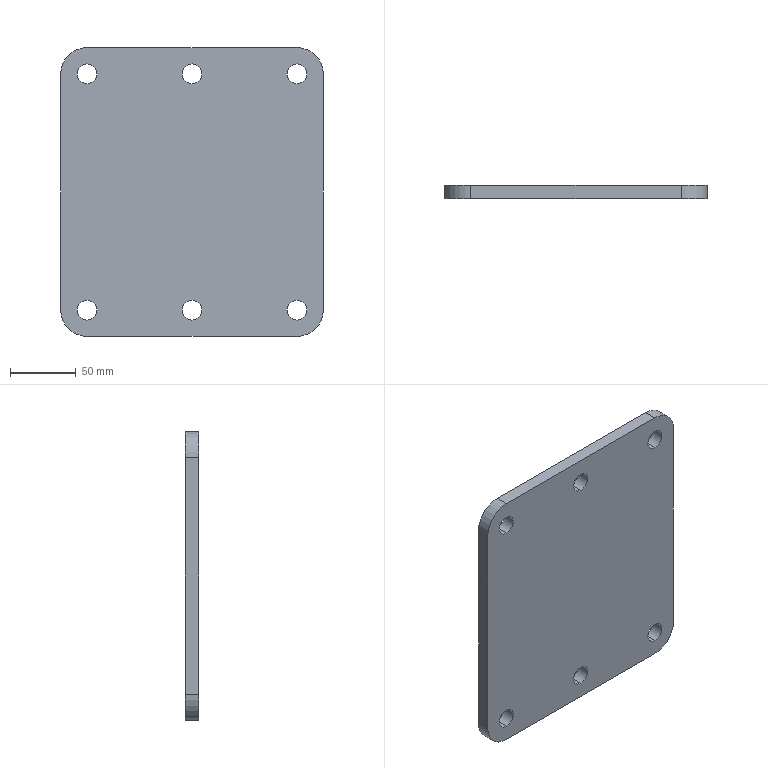Part | SolidWorks | features Extrusion 1, Fillet 1, ICE 1, LPattern 1 | 1 solid | 22 faces | box 200 x 10 x 220 mm | volume 425963 mm3 | cylinder 16 | plane 6 | commonest cylinder face diameters 15 x12 40 x4
STEP:
#1=CARTESIAN_POINT('',(80.,-5.,82.5));
#2=VERTEX_POINT('',#1);
#3=CARTESIAN_POINT('',(80.,-5.,97.5));
#4=VERTEX_POINT('',#3);
#5=CARTESIAN_POINT('',(80.,-5.,90.));
#6=DIRECTION('',(0.,1.,0.));
#7=DIRECTION('',(0.,0.,1.));
#8=AXIS2_PLACEMENT_3D('',#5,#6,#7);
#9=CIRCLE('',#8,7.5);
#10=EDGE_CURVE('',#2,#4,#9,.T.);
#11=ORIENTED_EDGE('',*,*,#10,.F.);
#12=CARTESIAN_POINT('',(80.,5.,82.5));
#13=VERTEX_POINT('',#12);
#14=CARTESIAN_POINT('',(80.,-5.,82.5));
#15=DIRECTION('',(0.,1.,0.));
#16=VECTOR('',#15,1000.);
#17=LINE('',#14,#16);
#18=EDGE_CURVE('',#2,#13,#17,.T.);
#19=ORIENTED_EDGE('',*,*,#18,.T.);
#20=CARTESIAN_POINT('',(80.,5.,97.5));
#21=VERTEX_POINT('',#20);
#22=CARTESIAN_POINT('',(80.,5.,90.));
#23=DIRECTION('',(0.,1.,0.));
#24=DIRECTION('',(0.,0.,1.));
#25=AXIS2_PLACEMENT_3D('',#22,#23,#24);
#26=CIRCLE('',#25,7.5);
#27=EDGE_CURVE('',#13,#21,#26,.T.);
#28=ORIENTED_EDGE('',*,*,#27,.T.);
#29=CARTESIAN_POINT('',(80.,-5.,97.5));
#30=DIRECTION('',(0.,1.,0.));
#31=VECTOR('',#30,1000.);
#32=LINE('',#29,#31);
#33=EDGE_CURVE('',#4,#21,#32,.T.);
#34=ORIENTED_EDGE('',*,*,#33,.F.);
#35=EDGE_LOOP('',(#11,#19,#28,#34));
#36=FACE_OUTER_BOUND('',#35,.T.);
#37=CARTESIAN_POINT('',(80.,-5.,90.));
#38=DIRECTION('',(0.,1.,0.));
#39=DIRECTION('',(0.,0.,1.));
#40=AXIS2_PLACEMENT_3D('',#37,#38,#39);
#41=CYLINDRICAL_SURFACE('',#40,7.5);
#42=ADVANCED_FACE('',(#36),#41,.F.);
#43=CARTESIAN_POINT('',(80.,-5.,-97.5));
#44=VERTEX_POINT('',#43);
#45=CARTESIAN_POINT('',(80.,-5.,-82.5));
#46=VERTEX_POINT('',#45);
#47=CARTESIAN_POINT('',(80.,-5.,-90.));
#48=DIRECTION('',(0.,1.,0.));
#49=DIRECTION('',(0.,0.,1.));
#50=AXIS2_PLACEMENT_3D('',#47,#48,#49);
#51=CIRCLE('',#50,7.5);
#52=EDGE_CURVE('',#44,#46,#51,.T.);
#53=ORIENTED_EDGE('',*,*,#52,.F.);
#54=CARTESIAN_POINT('',(80.,5.,-97.5));
#55=VERTEX_POINT('',#54);
#56=CARTESIAN_POINT('',(80.,-5.,-97.5));
#57=DIRECTION('',(0.,1.,0.));
#58=VECTOR('',#57,1000.);
#59=LINE('',#56,#58);
#60=EDGE_CURVE('',#44,#55,#59,.T.);
#61=ORIENTED_EDGE('',*,*,#60,.T.);
#62=CARTESIAN_POINT('',(80.,5.,-82.5));
#63=VERTEX_POINT('',#62);
#64=CARTESIAN_POINT('',(80.,5.,-90.));
#65=DIRECTION('',(0.,1.,0.));
#66=DIRECTION('',(0.,0.,1.));
#67=AXIS2_PLACEMENT_3D('',#64,#65,#66);
#68=CIRCLE('',#67,7.5);
#69=EDGE_CURVE('',#55,#63,#68,.T.);
#70=ORIENTED_EDGE('',*,*,#69,.T.);
#71=CARTESIAN_POINT('',(80.,-5.,-82.5));
#72=DIRECTION('',(0.,1.,0.));
#73=VECTOR('',#72,1000.);
#74=LINE('',#71,#73);
#75=EDGE_CURVE('',#46,#63,#74,.T.);
#76=ORIENTED_EDGE('',*,*,#75,.F.);
#77=EDGE_LOOP('',(#53,#61,#70,#76));
#78=FACE_OUTER_BOUND('',#77,.T.);
#79=CARTESIAN_POINT('',(80.,-5.,-90.));
#80=DIRECTION('',(0.,1.,0.));
#81=DIRECTION('',(0.,0.,1.));
#82=AXIS2_PLACEMENT_3D('',#79,#80,#81);
#83=CYLINDRICAL_SURFACE('',#82,7.5);
#84=ADVANCED_FACE('',(#78),#83,.F.);
#85=CARTESIAN_POINT('',(0.,-5.,-97.5));
#86=VERTEX_POINT('',#85);
#87=CARTESIAN_POINT('',(0.,-5.,-82.5));
#88=VERTEX_POINT('',#87);
#89=CARTESIAN_POINT('',(0.,-5.,-90.));
#90=DIRECTION('',(0.,1.,0.));
#91=DIRECTION('',(0.,0.,1.));
#92=AXIS2_PLACEMENT_3D('',#89,#90,#91);
#93=CIRCLE('',#92,7.5);
#94=EDGE_CURVE('',#86,#88,#93,.T.);
#95=ORIENTED_EDGE('',*,*,#94,.F.);
#96=CARTESIAN_POINT('',(0.,5.,-97.5));
#97=VERTEX_POINT('',#96);
#98=CARTESIAN_POINT('',(0.,-5.,-97.5));
#99=DIRECTION('',(0.,1.,0.));
#100=VECTOR('',#99,1000.);
#101=LINE('',#98,#100);
#102=EDGE_CURVE('',#86,#97,#101,.T.);
#103=ORIENTED_EDGE('',*,*,#102,.T.);
#104=CARTESIAN_POINT('',(0.,5.,-82.5));
#105=VERTEX_POINT('',#104);
#106=CARTESIAN_POINT('',(0.,5.,-90.));
#107=DIRECTION('',(0.,1.,0.));
#108=DIRECTION('',(0.,0.,1.));
#109=AXIS2_PLACEMENT_3D('',#106,#107,#108);
#110=CIRCLE('',#109,7.5);
#111=EDGE_CURVE('',#97,#105,#110,.T.);
#112=ORIENTED_EDGE('',*,*,#111,.T.);
#113=CARTESIAN_POINT('',(0.,-5.,-82.5));
#114=DIRECTION('',(0.,1.,0.));
#115=VECTOR('',#114,1000.);
#116=LINE('',#113,#115);
#117=EDGE_CURVE('',#88,#105,#116,.T.);
#118=ORIENTED_EDGE('',*,*,#117,.F.);
#119=EDGE_LOOP('',(#95,#103,#112,#118));
#120=FACE_OUTER_BOUND('',#119,.T.);
#121=CARTESIAN_POINT('',(0.,-5.,-90.));
#122=DIRECTION('',(0.,1.,0.));
#123=DIRECTION('',(0.,0.,1.));
#124=AXIS2_PLACEMENT_3D('',#121,#122,#123);
#125=CYLINDRICAL_SURFACE('',#124,7.5);
#126=ADVANCED_FACE('',(#120),#125,.F.);
#127=CARTESIAN_POINT('',(0.,-5.,82.5));
#128=VERTEX_POINT('',#127);
#129=CARTESIAN_POINT('',(0.,-5.,97.5));
#130=VERTEX_POINT('',#129);
#131=CARTESIAN_POINT('',(0.,-5.,90.));
#132=DIRECTION('',(0.,1.,0.));
#133=DIRECTION('',(0.,0.,1.));
#134=AXIS2_PLACEMENT_3D('',#131,#132,#133);
#135=CIRCLE('',#134,7.5);
#136=EDGE_CURVE('',#128,#130,#135,.T.);
#137=ORIENTED_EDGE('',*,*,#136,.F.);
#138=CARTESIAN_POINT('',(0.,5.,82.5));
#139=VERTEX_POINT('',#138);
#140=CARTESIAN_POINT('',(0.,-5.,82.5));
#141=DIRECTION('',(0.,1.,0.));
#142=VECTOR('',#141,1000.);
#143=LINE('',#140,#142);
#144=EDGE_CURVE('',#128,#139,#143,.T.);
#145=ORIENTED_EDGE('',*,*,#144,.T.);
#146=CARTESIAN_POINT('',(0.,5.,97.5));
#147=VERTEX_POINT('',#146);
#148=CARTESIAN_POINT('',(0.,5.,90.));
#149=DIRECTION('',(0.,1.,0.));
#150=DIRECTION('',(0.,0.,1.));
#151=AXIS2_PLACEMENT_3D('',#148,#149,#150);
#152=CIRCLE('',#151,7.5);
#153=EDGE_CURVE('',#139,#147,#152,.T.);
#154=ORIENTED_EDGE('',*,*,#153,.T.);
#155=CARTESIAN_POINT('',(0.,-5.,97.5));
#156=DIRECTION('',(0.,1.,0.));
#157=VECTOR('',#156,1000.);
#158=LINE('',#155,#157);
#159=EDGE_CURVE('',#130,#147,#158,.T.);
#160=ORIENTED_EDGE('',*,*,#159,.F.);
#161=EDGE_LOOP('',(#137,#145,#154,#160));
#162=FACE_OUTER_BOUND('',#161,.T.);
#163=CARTESIAN_POINT('',(0.,-5.,90.));
#164=DIRECTION('',(0.,1.,0.));
#165=DIRECTION('',(0.,0.,1.));
#166=AXIS2_PLACEMENT_3D('',#163,#164,#165);
#167=CYLINDRICAL_SURFACE('',#166,7.5);
#168=ADVANCED_FACE('',(#162),#167,.F.);
#169=CARTESIAN_POINT('',(-80.,-5.,-97.5));
#170=VERTEX_POINT('',#169);
#171=CARTESIAN_POINT('',(-80.,-5.,-82.5));
#172=VERTEX_POINT('',#171);
#173=CARTESIAN_POINT('',(-80.,-5.,-90.));
#174=DIRECTION('',(0.,1.,0.));
#175=DIRECTION('',(0.,0.,1.));
#176=AXIS2_PLACEMENT_3D('',#173,#174,#175);
#177=CIRCLE('',#176,7.5);
#178=EDGE_CURVE('',#170,#172,#177,.T.);
#179=ORIENTED_EDGE('',*,*,#178,.F.);
#180=CARTESIAN_POINT('',(-80.,5.,-97.5));
#181=VERTEX_POINT('',#180);
#182=CARTESIAN_POINT('',(-80.,-5.,-97.5));
#183=DIRECTION('',(0.,1.,0.));
#184=VECTOR('',#183,1000.);
#185=LINE('',#182,#184);
#186=EDGE_CURVE('',#170,#181,#185,.T.);
#187=ORIENTED_EDGE('',*,*,#186,.T.);
#188=CARTESIAN_POINT('',(-80.,5.,-82.5));
#189=VERTEX_POINT('',#188);
#190=CARTESIAN_POINT('',(-80.,5.,-90.));
#191=DIRECTION('',(0.,1.,0.));
#192=DIRECTION('',(0.,0.,1.));
#193=AXIS2_PLACEMENT_3D('',#190,#191,#192);
#194=CIRCLE('',#193,7.5);
#195=EDGE_CURVE('',#181,#189,#194,.T.);
#196=ORIENTED_EDGE('',*,*,#195,.T.);
#197=CARTESIAN_POINT('',(-80.,-5.,-82.5));
#198=DIRECTION('',(0.,1.,0.));
#199=VECTOR('',#198,1000.);
#200=LINE('',#197,#199);
#201=EDGE_CURVE('',#172,#189,#200,.T.);
#202=ORIENTED_EDGE('',*,*,#201,.F.);
#203=EDGE_LOOP('',(#179,#187,#196,#202));
#204=FACE_OUTER_BOUND('',#203,.T.);
#205=CARTESIAN_POINT('',(-80.,-5.,-90.));
#206=DIRECTION('',(0.,1.,0.));
#207=DIRECTION('',(0.,0.,1.));
#208=AXIS2_PLACEMENT_3D('',#205,#206,#207);
#209=CYLINDRICAL_SURFACE('',#208,7.5);
#210=ADVANCED_FACE('',(#204),#209,.F.);
#211=CARTESIAN_POINT('',(-80.,-5.,82.5));
#212=VERTEX_POINT('',#211);
#213=CARTESIAN_POINT('',(-80.,-5.,97.5));
#214=VERTEX_POINT('',#213);
#215=CARTESIAN_POINT('',(-80.,-5.,90.));
#216=DIRECTION('',(0.,1.,0.));
#217=DIRECTION('',(0.,0.,1.));
#218=AXIS2_PLACEMENT_3D('',#215,#216,#217);
#219=CIRCLE('',#218,7.5);
#220=EDGE_CURVE('',#212,#214,#219,.T.);
#221=ORIENTED_EDGE('',*,*,#220,.F.);
#222=CARTESIAN_POINT('',(-80.,5.,82.5));
#223=VERTEX_POINT('',#222);
#224=CARTESIAN_POINT('',(-80.,-5.,82.5));
#225=DIRECTION('',(0.,1.,0.));
#226=VECTOR('',#225,1000.);
#227=LINE('',#224,#226);
#228=EDGE_CURVE('',#212,#223,#227,.T.);
#229=ORIENTED_EDGE('',*,*,#228,.T.);
#230=CARTESIAN_POINT('',(-80.,5.,97.5));
#231=VERTEX_POINT('',#230);
#232=CARTESIAN_POINT('',(-80.,5.,90.));
#233=DIRECTION('',(0.,1.,0.));
#234=DIRECTION('',(0.,0.,1.));
#235=AXIS2_PLACEMENT_3D('',#232,#233,#234);
#236=CIRCLE('',#235,7.5);
#237=EDGE_CURVE('',#223,#231,#236,.T.);
#238=ORIENTED_EDGE('',*,*,#237,.T.);
#239=CARTESIAN_POINT('',(-80.,-5.,97.5));
#240=DIRECTION('',(0.,1.,0.));
#241=VECTOR('',#240,1000.);
#242=LINE('',#239,#241);
#243=EDGE_CURVE('',#214,#231,#242,.T.);
#244=ORIENTED_EDGE('',*,*,#243,.F.);
#245=EDGE_LOOP('',(#221,#229,#238,#244));
#246=FACE_OUTER_BOUND('',#245,.T.);
#247=CARTESIAN_POINT('',(-80.,-5.,90.));
#248=DIRECTION('',(0.,1.,0.));
#249=DIRECTION('',(0.,0.,1.));
#250=AXIS2_PLACEMENT_3D('',#247,#248,#249);
#251=CYLINDRICAL_SURFACE('',#250,7.5);
#252=ADVANCED_FACE('',(#246),#251,.F.);
#253=ORIENTED_EDGE('',*,*,#228,.F.);
#254=CARTESIAN_POINT('',(-80.,-5.,90.));
#255=DIRECTION('',(0.,1.,0.));
#256=DIRECTION('',(0.,0.,1.));
#257=AXIS2_PLACEMENT_3D('',#254,#255,#256);
#258=CIRCLE('',#257,7.5);
#259=EDGE_CURVE('',#214,#212,#258,.T.);
#260=ORIENTED_EDGE('',*,*,#259,.F.);
#261=ORIENTED_EDGE('',*,*,#243,.T.);
#262=CARTESIAN_POINT('',(-80.,5.,90.));
#263=DIRECTION('',(0.,1.,0.));
#264=DIRECTION('',(0.,0.,1.));
#265=AXIS2_PLACEMENT_3D('',#262,#263,#264);
#266=CIRCLE('',#265,7.5);
#267=EDGE_CURVE('',#231,#223,#266,.T.);
#268=ORIENTED_EDGE('',*,*,#267,.T.);
#269=EDGE_LOOP('',(#253,#260,#261,#268));
#270=FACE_OUTER_BOUND('',#269,.T.);
#271=CARTESIAN_POINT('',(-80.,-5.,90.));
#272=DIRECTION('',(0.,1.,0.));
#273=DIRECTION('',(0.,0.,1.));
#274=AXIS2_PLACEMENT_3D('',#271,#272,#273);
#275=CYLINDRICAL_SURFACE('',#274,7.5);
#276=ADVANCED_FACE('',(#270),#275,.F.);
#277=ORIENTED_EDGE('',*,*,#186,.F.);
#278=CARTESIAN_POINT('',(-80.,-5.,-90.));
#279=DIRECTION('',(0.,1.,0.));
#280=DIRECTION('',(0.,0.,1.));
#281=AXIS2_PLACEMENT_3D('',#278,#279,#280);
#282=CIRCLE('',#281,7.5);
#283=EDGE_CURVE('',#172,#170,#282,.T.);
#284=ORIENTED_EDGE('',*,*,#283,.F.);
#285=ORIENTED_EDGE('',*,*,#201,.T.);
#286=CARTESIAN_POINT('',(-80.,5.,-90.));
#287=DIRECTION('',(0.,1.,0.));
#288=DIRECTION('',(0.,0.,1.));
#289=AXIS2_PLACEMENT_3D('',#286,#287,#288);
#290=CIRCLE('',#289,7.5);
#291=EDGE_CURVE('',#189,#181,#290,.T.);
#292=ORIENTED_EDGE('',*,*,#291,.T.);
#293=EDGE_LOOP('',(#277,#284,#285,#292));
#294=FACE_OUTER_BOUND('',#293,.T.);
#295=CARTESIAN_POINT('',(-80.,-5.,-90.));
#296=DIRECTION('',(0.,1.,0.));
#297=DIRECTION('',(0.,0.,1.));
#298=AXIS2_PLACEMENT_3D('',#295,#296,#297);
#299=CYLINDRICAL_SURFACE('',#298,7.5);
#300=ADVANCED_FACE('',(#294),#299,.F.);
#301=ORIENTED_EDGE('',*,*,#144,.F.);
#302=CARTESIAN_POINT('',(0.,-5.,90.));
#303=DIRECTION('',(0.,1.,0.));
#304=DIRECTION('',(0.,0.,1.));
#305=AXIS2_PLACEMENT_3D('',#302,#303,#304);
#306=CIRCLE('',#305,7.5);
#307=EDGE_CURVE('',#130,#128,#306,.T.);
#308=ORIENTED_EDGE('',*,*,#307,.F.);
#309=ORIENTED_EDGE('',*,*,#159,.T.);
#310=CARTESIAN_POINT('',(0.,5.,90.));
#311=DIRECTION('',(0.,1.,0.));
#312=DIRECTION('',(0.,0.,1.));
#313=AXIS2_PLACEMENT_3D('',#310,#311,#312);
#314=CIRCLE('',#313,7.5);
#315=EDGE_CURVE('',#147,#139,#314,.T.);
#316=ORIENTED_EDGE('',*,*,#315,.T.);
#317=EDGE_LOOP('',(#301,#308,#309,#316));
#318=FACE_OUTER_BOUND('',#317,.T.);
#319=CARTESIAN_POINT('',(0.,-5.,90.));
#320=DIRECTION('',(0.,1.,0.));
#321=DIRECTION('',(0.,0.,1.));
#322=AXIS2_PLACEMENT_3D('',#319,#320,#321);
#323=CYLINDRICAL_SURFACE('',#322,7.5);
#324=ADVANCED_FACE('',(#318),#323,.F.);
#325=ORIENTED_EDGE('',*,*,#102,.F.);
#326=CARTESIAN_POINT('',(0.,-5.,-90.));
#327=DIRECTION('',(0.,1.,0.));
#328=DIRECTION('',(0.,0.,1.));
#329=AXIS2_PLACEMENT_3D('',#326,#327,#328);
#330=CIRCLE('',#329,7.5);
#331=EDGE_CURVE('',#88,#86,#330,.T.);
#332=ORIENTED_EDGE('',*,*,#331,.F.);
#333=ORIENTED_EDGE('',*,*,#117,.T.);
#334=CARTESIAN_POINT('',(0.,5.,-90.));
#335=DIRECTION('',(0.,1.,0.));
#336=DIRECTION('',(0.,0.,1.));
#337=AXIS2_PLACEMENT_3D('',#334,#335,#336);
#338=CIRCLE('',#337,7.5);
#339=EDGE_CURVE('',#105,#97,#338,.T.);
#340=ORIENTED_EDGE('',*,*,#339,.T.);
#341=EDGE_LOOP('',(#325,#332,#333,#340));
#342=FACE_OUTER_BOUND('',#341,.T.);
#343=CARTESIAN_POINT('',(0.,-5.,-90.));
#344=DIRECTION('',(0.,1.,0.));
#345=DIRECTION('',(0.,0.,1.));
#346=AXIS2_PLACEMENT_3D('',#343,#344,#345);
#347=CYLINDRICAL_SURFACE('',#346,7.5);
#348=ADVANCED_FACE('',(#342),#347,.F.);
#349=CARTESIAN_POINT('',(100.,5.,90.));
#350=VERTEX_POINT('',#349);
#351=CARTESIAN_POINT('',(100.,5.,-90.));
#352=VERTEX_POINT('',#351);
#353=CARTESIAN_POINT('',(100.,5.,-110.));
#354=DIRECTION('',(0.,0.,-1.));
#355=VECTOR('',#354,1000.);
#356=LINE('',#353,#355);
#357=EDGE_CURVE('',#350,#352,#356,.T.);
#358=ORIENTED_EDGE('',*,*,#357,.F.);
#359=CARTESIAN_POINT('',(100.,-5.,90.));
#360=VERTEX_POINT('',#359);
#361=CARTESIAN_POINT('',(100.,5.,90.));
#362=DIRECTION('',(0.,-1.,0.));
#363=VECTOR('',#362,1000.);
#364=LINE('',#361,#363);
#365=EDGE_CURVE('',#350,#360,#364,.T.);
#366=ORIENTED_EDGE('',*,*,#365,.T.);
#367=CARTESIAN_POINT('',(100.,-5.,-90.));
#368=VERTEX_POINT('',#367);
#369=CARTESIAN_POINT('',(100.,-5.,-110.));
#370=DIRECTION('',(0.,0.,-1.));
#371=VECTOR('',#370,1000.);
#372=LINE('',#369,#371);
#373=EDGE_CURVE('',#360,#368,#372,.T.);
#374=ORIENTED_EDGE('',*,*,#373,.T.);
#375=CARTESIAN_POINT('',(100.,5.,-90.));
#376=DIRECTION('',(0.,1.,0.));
#377=VECTOR('',#376,1000.);
#378=LINE('',#375,#377);
#379=EDGE_CURVE('',#368,#352,#378,.T.);
#380=ORIENTED_EDGE('',*,*,#379,.T.);
#381=EDGE_LOOP('',(#358,#366,#374,#380));
#382=FACE_OUTER_BOUND('',#381,.T.);
#383=CARTESIAN_POINT('',(100.,5.,-110.));
#384=DIRECTION('',(-1.,0.,0.));
#385=DIRECTION('',(0.,0.,1.));
#386=AXIS2_PLACEMENT_3D('',#383,#384,#385);
#387=PLANE('',#386);
#388=ADVANCED_FACE('',(#382),#387,.F.);
#389=CARTESIAN_POINT('',(80.,-5.,-110.));
#390=VERTEX_POINT('',#389);
#391=CARTESIAN_POINT('',(-80.,-5.,-110.));
#392=VERTEX_POINT('',#391);
#393=CARTESIAN_POINT('',(-100.,-5.,-110.));
#394=DIRECTION('',(-1.,0.,0.));
#395=VECTOR('',#394,1000.);
#396=LINE('',#393,#395);
#397=EDGE_CURVE('',#390,#392,#396,.T.);
#398=ORIENTED_EDGE('',*,*,#397,.T.);
#399=CARTESIAN_POINT('',(-80.,5.,-110.));
#400=VERTEX_POINT('',#399);
#401=CARTESIAN_POINT('',(-80.,5.,-110.));
#402=DIRECTION('',(0.,1.,0.));
#403=VECTOR('',#402,1000.);
#404=LINE('',#401,#403);
#405=EDGE_CURVE('',#392,#400,#404,.T.);
#406=ORIENTED_EDGE('',*,*,#405,.T.);
#407=CARTESIAN_POINT('',(80.,5.,-110.));
#408=VERTEX_POINT('',#407);
#409=CARTESIAN_POINT('',(-100.,5.,-110.));
#410=DIRECTION('',(-1.,0.,0.));
#411=VECTOR('',#410,1000.);
#412=LINE('',#409,#411);
#413=EDGE_CURVE('',#408,#400,#412,.T.);
#414=ORIENTED_EDGE('',*,*,#413,.F.);
#415=CARTESIAN_POINT('',(80.,5.,-110.));
#416=DIRECTION('',(0.,-1.,0.));
#417=VECTOR('',#416,1000.);
#418=LINE('',#415,#417);
#419=EDGE_CURVE('',#408,#390,#418,.T.);
#420=ORIENTED_EDGE('',*,*,#419,.T.);
#421=EDGE_LOOP('',(#398,#406,#414,#420));
#422=FACE_OUTER_BOUND('',#421,.T.);
#423=CARTESIAN_POINT('',(-100.,5.,-110.));
#424=DIRECTION('',(0.,0.,1.));
#425=DIRECTION('',(1.,0.,0.));
#426=AXIS2_PLACEMENT_3D('',#423,#424,#425);
#427=PLANE('',#426);
#428=ADVANCED_FACE('',(#422),#427,.F.);
#429=CARTESIAN_POINT('',(-100.,5.,-90.));
#430=VERTEX_POINT('',#429);
#431=CARTESIAN_POINT('',(-100.,5.,90.));
#432=VERTEX_POINT('',#431);
#433=CARTESIAN_POINT('',(-100.,5.,-110.));
#434=DIRECTION('',(0.,0.,1.));
#435=VECTOR('',#434,1000.);
#436=LINE('',#433,#435);
#437=EDGE_CURVE('',#430,#432,#436,.T.);
#438=ORIENTED_EDGE('',*,*,#437,.F.);
#439=CARTESIAN_POINT('',(-100.,-5.,-90.));
#440=VERTEX_POINT('',#439);
#441=CARTESIAN_POINT('',(-100.,5.,-90.));
#442=DIRECTION('',(0.,-1.,0.));
#443=VECTOR('',#442,1000.);
#444=LINE('',#441,#443);
#445=EDGE_CURVE('',#430,#440,#444,.T.);
#446=ORIENTED_EDGE('',*,*,#445,.T.);
#447=CARTESIAN_POINT('',(-100.,-5.,90.));
#448=VERTEX_POINT('',#447);
#449=CARTESIAN_POINT('',(-100.,-5.,-110.));
#450=DIRECTION('',(0.,0.,1.));
#451=VECTOR('',#450,1000.);
#452=LINE('',#449,#451);
#453=EDGE_CURVE('',#440,#448,#452,.T.);
#454=ORIENTED_EDGE('',*,*,#453,.T.);
#455=CARTESIAN_POINT('',(-100.,5.,90.));
#456=DIRECTION('',(0.,1.,0.));
#457=VECTOR('',#456,1000.);
#458=LINE('',#455,#457);
#459=EDGE_CURVE('',#448,#432,#458,.T.);
#460=ORIENTED_EDGE('',*,*,#459,.T.);
#461=EDGE_LOOP('',(#438,#446,#454,#460));
#462=FACE_OUTER_BOUND('',#461,.T.);
#463=CARTESIAN_POINT('',(-100.,5.,-110.));
#464=DIRECTION('',(1.,0.,0.));
#465=DIRECTION('',(0.,0.,-1.));
#466=AXIS2_PLACEMENT_3D('',#463,#464,#465);
#467=PLANE('',#466);
#468=ADVANCED_FACE('',(#462),#467,.F.);
#469=CARTESIAN_POINT('',(-80.,5.,110.));
#470=VERTEX_POINT('',#469);
#471=CARTESIAN_POINT('',(80.,5.,110.));
#472=VERTEX_POINT('',#471);
#473=CARTESIAN_POINT('',(-100.,5.,110.));
#474=DIRECTION('',(1.,0.,0.));
#475=VECTOR('',#474,1000.);
#476=LINE('',#473,#475);
#477=EDGE_CURVE('',#470,#472,#476,.T.);
#478=ORIENTED_EDGE('',*,*,#477,.F.);
#479=CARTESIAN_POINT('',(-80.,-5.,110.));
#480=VERTEX_POINT('',#479);
#481=CARTESIAN_POINT('',(-80.,5.,110.));
#482=DIRECTION('',(0.,-1.,0.));
#483=VECTOR('',#482,1000.);
#484=LINE('',#481,#483);
#485=EDGE_CURVE('',#470,#480,#484,.T.);
#486=ORIENTED_EDGE('',*,*,#485,.T.);
#487=CARTESIAN_POINT('',(80.,-5.,110.));
#488=VERTEX_POINT('',#487);
#489=CARTESIAN_POINT('',(-100.,-5.,110.));
#490=DIRECTION('',(1.,0.,0.));
#491=VECTOR('',#490,1000.);
#492=LINE('',#489,#491);
#493=EDGE_CURVE('',#480,#488,#492,.T.);
#494=ORIENTED_EDGE('',*,*,#493,.T.);
#495=CARTESIAN_POINT('',(80.,5.,110.));
#496=DIRECTION('',(0.,1.,0.));
#497=VECTOR('',#496,1000.);
#498=LINE('',#495,#497);
#499=EDGE_CURVE('',#488,#472,#498,.T.);
#500=ORIENTED_EDGE('',*,*,#499,.T.);
#501=EDGE_LOOP('',(#478,#486,#494,#500));
#502=FACE_OUTER_BOUND('',#501,.T.);
#503=CARTESIAN_POINT('',(-100.,5.,110.));
#504=DIRECTION('',(0.,0.,-1.));
#505=DIRECTION('',(-1.,0.,0.));
#506=AXIS2_PLACEMENT_3D('',#503,#504,#505);
#507=PLANE('',#506);
#508=ADVANCED_FACE('',(#502),#507,.F.);
#509=CARTESIAN_POINT('',(80.,5.,90.));
#510=DIRECTION('',(0.,1.,0.));
#511=DIRECTION('',(0.,0.,1.));
#512=AXIS2_PLACEMENT_3D('',#509,#510,#511);
#513=CIRCLE('',#512,7.5);
#514=EDGE_CURVE('',#21,#13,#513,.T.);
#515=ORIENTED_EDGE('',*,*,#514,.F.);
#516=ORIENTED_EDGE('',*,*,#27,.F.);
#517=EDGE_LOOP('',(#515,#516));
#518=FACE_BOUND('',#517,.T.);
#519=CARTESIAN_POINT('',(80.,5.,-90.));
#520=DIRECTION('',(0.,1.,0.));
#521=DIRECTION('',(0.,0.,1.));
#522=AXIS2_PLACEMENT_3D('',#519,#520,#521);
#523=CIRCLE('',#522,7.5);
#524=EDGE_CURVE('',#63,#55,#523,.T.);
#525=ORIENTED_EDGE('',*,*,#524,.F.);
#526=ORIENTED_EDGE('',*,*,#69,.F.);
#527=EDGE_LOOP('',(#525,#526));
#528=FACE_BOUND('',#527,.T.);
#529=ORIENTED_EDGE('',*,*,#413,.T.);
#530=CARTESIAN_POINT('',(-80.,5.,-90.));
#531=DIRECTION('',(0.,1.,0.));
#532=DIRECTION('',(0.,0.,1.));
#533=AXIS2_PLACEMENT_3D('',#530,#531,#532);
#534=CIRCLE('',#533,20.);
#535=EDGE_CURVE('',#400,#430,#534,.T.);
#536=ORIENTED_EDGE('',*,*,#535,.T.);
#537=ORIENTED_EDGE('',*,*,#437,.T.);
#538=CARTESIAN_POINT('',(-80.,5.,90.));
#539=DIRECTION('',(0.,1.,0.));
#540=DIRECTION('',(0.,0.,1.));
#541=AXIS2_PLACEMENT_3D('',#538,#539,#540);
#542=CIRCLE('',#541,20.);
#543=EDGE_CURVE('',#432,#470,#542,.T.);
#544=ORIENTED_EDGE('',*,*,#543,.T.);
#545=ORIENTED_EDGE('',*,*,#477,.T.);
#546=CARTESIAN_POINT('',(80.,5.,90.));
#547=DIRECTION('',(0.,1.,0.));
#548=DIRECTION('',(0.,0.,1.));
#549=AXIS2_PLACEMENT_3D('',#546,#547,#548);
#550=CIRCLE('',#549,20.);
#551=EDGE_CURVE('',#472,#350,#550,.T.);
#552=ORIENTED_EDGE('',*,*,#551,.T.);
#553=ORIENTED_EDGE('',*,*,#357,.T.);
#554=CARTESIAN_POINT('',(80.,5.,-90.));
#555=DIRECTION('',(0.,1.,0.));
#556=DIRECTION('',(0.,0.,1.));
#557=AXIS2_PLACEMENT_3D('',#554,#555,#556);
#558=CIRCLE('',#557,20.);
#559=EDGE_CURVE('',#352,#408,#558,.T.);
#560=ORIENTED_EDGE('',*,*,#559,.T.);
#561=EDGE_LOOP('',(#529,#536,#537,#544,#545,#552,#553,#560));
#562=FACE_OUTER_BOUND('',#561,.T.);
#563=ORIENTED_EDGE('',*,*,#339,.F.);
#564=ORIENTED_EDGE('',*,*,#111,.F.);
#565=EDGE_LOOP('',(#563,#564));
#566=FACE_BOUND('',#565,.T.);
#567=ORIENTED_EDGE('',*,*,#315,.F.);
#568=ORIENTED_EDGE('',*,*,#153,.F.);
#569=EDGE_LOOP('',(#567,#568));
#570=FACE_BOUND('',#569,.T.);
#571=ORIENTED_EDGE('',*,*,#291,.F.);
#572=ORIENTED_EDGE('',*,*,#195,.F.);
#573=EDGE_LOOP('',(#571,#572));
#574=FACE_BOUND('',#573,.T.);
#575=ORIENTED_EDGE('',*,*,#267,.F.);
#576=ORIENTED_EDGE('',*,*,#237,.F.);
#577=EDGE_LOOP('',(#575,#576));
#578=FACE_BOUND('',#577,.T.);
#579=CARTESIAN_POINT('',(0.,5.,0.));
#580=DIRECTION('',(0.,1.,0.));
#581=DIRECTION('',(0.,0.,1.));
#582=AXIS2_PLACEMENT_3D('',#579,#580,#581);
#583=PLANE('',#582);
#584=ADVANCED_FACE('',(#518,#528,#562,#566,#570,#574,#578),#583,.T.);
#585=CARTESIAN_POINT('',(80.,-5.,90.));
#586=DIRECTION('',(0.,1.,0.));
#587=DIRECTION('',(0.,0.,1.));
#588=AXIS2_PLACEMENT_3D('',#585,#586,#587);
#589=CIRCLE('',#588,7.5);
#590=EDGE_CURVE('',#4,#2,#589,.T.);
#591=ORIENTED_EDGE('',*,*,#590,.T.);
#592=ORIENTED_EDGE('',*,*,#10,.T.);
#593=EDGE_LOOP('',(#591,#592));
#594=FACE_BOUND('',#593,.T.);
#595=CARTESIAN_POINT('',(80.,-5.,-90.));
#596=DIRECTION('',(0.,1.,0.));
#597=DIRECTION('',(0.,0.,1.));
#598=AXIS2_PLACEMENT_3D('',#595,#596,#597);
#599=CIRCLE('',#598,7.5);
#600=EDGE_CURVE('',#46,#44,#599,.T.);
#601=ORIENTED_EDGE('',*,*,#600,.T.);
#602=ORIENTED_EDGE('',*,*,#52,.T.);
#603=EDGE_LOOP('',(#601,#602));
#604=FACE_BOUND('',#603,.T.);
#605=ORIENTED_EDGE('',*,*,#453,.F.);
#606=CARTESIAN_POINT('',(-80.,-5.,-90.));
#607=DIRECTION('',(0.,-1.,0.));
#608=DIRECTION('',(0.,0.,1.));
#609=AXIS2_PLACEMENT_3D('',#606,#607,#608);
#610=CIRCLE('',#609,20.);
#611=EDGE_CURVE('',#440,#392,#610,.T.);
#612=ORIENTED_EDGE('',*,*,#611,.T.);
#613=ORIENTED_EDGE('',*,*,#397,.F.);
#614=CARTESIAN_POINT('',(80.,-5.,-90.));
#615=DIRECTION('',(0.,-1.,0.));
#616=DIRECTION('',(0.,0.,1.));
#617=AXIS2_PLACEMENT_3D('',#614,#615,#616);
#618=CIRCLE('',#617,20.);
#619=EDGE_CURVE('',#390,#368,#618,.T.);
#620=ORIENTED_EDGE('',*,*,#619,.T.);
#621=ORIENTED_EDGE('',*,*,#373,.F.);
#622=CARTESIAN_POINT('',(80.,-5.,90.));
#623=DIRECTION('',(0.,-1.,0.));
#624=DIRECTION('',(0.,0.,1.));
#625=AXIS2_PLACEMENT_3D('',#622,#623,#624);
#626=CIRCLE('',#625,20.);
#627=EDGE_CURVE('',#360,#488,#626,.T.);
#628=ORIENTED_EDGE('',*,*,#627,.T.);
#629=ORIENTED_EDGE('',*,*,#493,.F.);
#630=CARTESIAN_POINT('',(-80.,-5.,90.));
#631=DIRECTION('',(0.,-1.,0.));
#632=DIRECTION('',(0.,0.,1.));
#633=AXIS2_PLACEMENT_3D('',#630,#631,#632);
#634=CIRCLE('',#633,20.);
#635=EDGE_CURVE('',#480,#448,#634,.T.);
#636=ORIENTED_EDGE('',*,*,#635,.T.);
#637=EDGE_LOOP('',(#605,#612,#613,#620,#621,#628,#629,#636));
#638=FACE_OUTER_BOUND('',#637,.T.);
#639=ORIENTED_EDGE('',*,*,#331,.T.);
#640=ORIENTED_EDGE('',*,*,#94,.T.);
#641=EDGE_LOOP('',(#639,#640));
#642=FACE_BOUND('',#641,.T.);
#643=ORIENTED_EDGE('',*,*,#307,.T.);
#644=ORIENTED_EDGE('',*,*,#136,.T.);
#645=EDGE_LOOP('',(#643,#644));
#646=FACE_BOUND('',#645,.T.);
#647=ORIENTED_EDGE('',*,*,#283,.T.);
#648=ORIENTED_EDGE('',*,*,#178,.T.);
#649=EDGE_LOOP('',(#647,#648));
#650=FACE_BOUND('',#649,.T.);
#651=ORIENTED_EDGE('',*,*,#259,.T.);
#652=ORIENTED_EDGE('',*,*,#220,.T.);
#653=EDGE_LOOP('',(#651,#652));
#654=FACE_BOUND('',#653,.T.);
#655=CARTESIAN_POINT('',(0.,-5.,0.));
#656=DIRECTION('',(0.,1.,0.));
#657=DIRECTION('',(0.,0.,1.));
#658=AXIS2_PLACEMENT_3D('',#655,#656,#657);
#659=PLANE('',#658);
#660=ADVANCED_FACE('',(#594,#604,#638,#642,#646,#650,#654),#659,.F.);
#661=ORIENTED_EDGE('',*,*,#60,.F.);
#662=ORIENTED_EDGE('',*,*,#600,.F.);
#663=ORIENTED_EDGE('',*,*,#75,.T.);
#664=ORIENTED_EDGE('',*,*,#524,.T.);
#665=EDGE_LOOP('',(#661,#662,#663,#664));
#666=FACE_OUTER_BOUND('',#665,.T.);
#667=CARTESIAN_POINT('',(80.,-5.,-90.));
#668=DIRECTION('',(0.,1.,0.));
#669=DIRECTION('',(0.,0.,1.));
#670=AXIS2_PLACEMENT_3D('',#667,#668,#669);
#671=CYLINDRICAL_SURFACE('',#670,7.5);
#672=ADVANCED_FACE('',(#666),#671,.F.);
#673=ORIENTED_EDGE('',*,*,#18,.F.);
#674=ORIENTED_EDGE('',*,*,#590,.F.);
#675=ORIENTED_EDGE('',*,*,#33,.T.);
#676=ORIENTED_EDGE('',*,*,#514,.T.);
#677=EDGE_LOOP('',(#673,#674,#675,#676));
#678=FACE_OUTER_BOUND('',#677,.T.);
#679=CARTESIAN_POINT('',(80.,-5.,90.));
#680=DIRECTION('',(0.,1.,0.));
#681=DIRECTION('',(0.,0.,1.));
#682=AXIS2_PLACEMENT_3D('',#679,#680,#681);
#683=CYLINDRICAL_SURFACE('',#682,7.5);
#684=ADVANCED_FACE('',(#678),#683,.F.);
#685=ORIENTED_EDGE('',*,*,#535,.F.);
#686=ORIENTED_EDGE('',*,*,#405,.F.);
#687=ORIENTED_EDGE('',*,*,#611,.F.);
#688=ORIENTED_EDGE('',*,*,#445,.F.);
#689=EDGE_LOOP('',(#685,#686,#687,#688));
#690=FACE_OUTER_BOUND('',#689,.T.);
#691=CARTESIAN_POINT('',(-80.,5.,-90.));
#692=DIRECTION('',(0.,-1.,0.));
#693=DIRECTION('',(0.,0.,-1.));
#694=AXIS2_PLACEMENT_3D('',#691,#692,#693);
#695=CYLINDRICAL_SURFACE('',#694,20.);
#696=ADVANCED_FACE('',(#690),#695,.T.);
#697=ORIENTED_EDGE('',*,*,#543,.F.);
#698=ORIENTED_EDGE('',*,*,#459,.F.);
#699=ORIENTED_EDGE('',*,*,#635,.F.);
#700=ORIENTED_EDGE('',*,*,#485,.F.);
#701=EDGE_LOOP('',(#697,#698,#699,#700));
#702=FACE_OUTER_BOUND('',#701,.T.);
#703=CARTESIAN_POINT('',(-80.,5.,90.));
#704=DIRECTION('',(0.,-1.,0.));
#705=DIRECTION('',(0.,0.,-1.));
#706=AXIS2_PLACEMENT_3D('',#703,#704,#705);
#707=CYLINDRICAL_SURFACE('',#706,20.);
#708=ADVANCED_FACE('',(#702),#707,.T.);
#709=ORIENTED_EDGE('',*,*,#551,.F.);
#710=ORIENTED_EDGE('',*,*,#499,.F.);
#711=ORIENTED_EDGE('',*,*,#627,.F.);
#712=ORIENTED_EDGE('',*,*,#365,.F.);
#713=EDGE_LOOP('',(#709,#710,#711,#712));
#714=FACE_OUTER_BOUND('',#713,.T.);
#715=CARTESIAN_POINT('',(80.,5.,90.));
#716=DIRECTION('',(0.,-1.,0.));
#717=DIRECTION('',(0.,0.,-1.));
#718=AXIS2_PLACEMENT_3D('',#715,#716,#717);
#719=CYLINDRICAL_SURFACE('',#718,20.);
#720=ADVANCED_FACE('',(#714),#719,.T.);
#721=ORIENTED_EDGE('',*,*,#559,.F.);
#722=ORIENTED_EDGE('',*,*,#379,.F.);
#723=ORIENTED_EDGE('',*,*,#619,.F.);
#724=ORIENTED_EDGE('',*,*,#419,.F.);
#725=EDGE_LOOP('',(#721,#722,#723,#724));
#726=FACE_OUTER_BOUND('',#725,.T.);
#727=CARTESIAN_POINT('',(80.,5.,-90.));
#728=DIRECTION('',(0.,-1.,0.));
#729=DIRECTION('',(0.,0.,-1.));
#730=AXIS2_PLACEMENT_3D('',#727,#728,#729);
#731=CYLINDRICAL_SURFACE('',#730,20.);
#732=ADVANCED_FACE('',(#726),#731,.T.);
#733=CLOSED_SHELL('',(#42,#84,#126,#168,#210,#252,#276,#300,#324,#348,#388,#428,#468,#508,#584,#660,#672,#684,#696,#708,#720,#732));
#734=MANIFOLD_SOLID_BREP('',#733);
#735=CARTESIAN_POINT('',(0.,0.,0.));
#736=DIRECTION('',(0.,0.,1.));
#737=DIRECTION('',(1.,0.,0.));
#738=AXIS2_PLACEMENT_3D('',#735,#736,#737);
#739=(LENGTH_UNIT()NAMED_UNIT(*)SI_UNIT(.MILLI.,.METRE.));
#740=UNCERTAINTY_MEASURE_WITH_UNIT(LENGTH_MEASURE(0.00001),#739,'','');
#741=(NAMED_UNIT(*)PLANE_ANGLE_UNIT()SI_UNIT($,.RADIAN.));
#742=(NAMED_UNIT(*)SI_UNIT($,.STERADIAN.)SOLID_ANGLE_UNIT());
#743=(GEOMETRIC_REPRESENTATION_CONTEXT(3)GLOBAL_UNCERTAINTY_ASSIGNED_CONTEXT((#740))GLOBAL_UNIT_ASSIGNED_CONTEXT((#739,#741,#742))REPRESENTATION_CONTEXT('',''));
#744=ADVANCED_BREP_SHAPE_REPRESENTATION('',(#734,#738),#743);